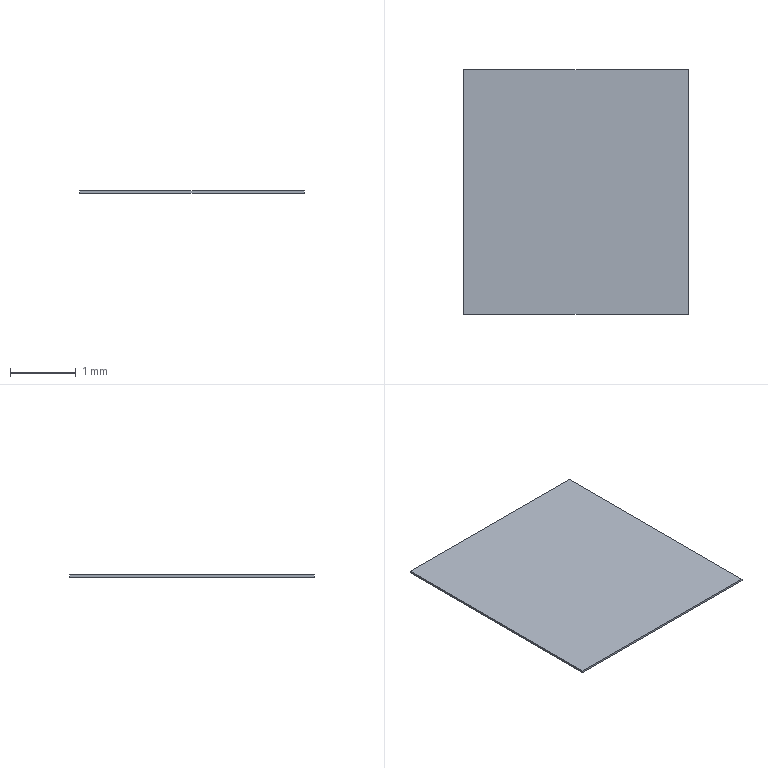Part | Creo | 1 solid | 6 faces | box 3.425 x 3.725 x 0.03048 mm | volume 0.389 mm3 | plane 6
STEP:
#1=CARTESIAN_POINT('',(0.,0.,0.));
#2=DIRECTION('',(0.,0.,1.));
#3=DIRECTION('',(1.,0.,0.));
#4=AXIS2_PLACEMENT_3D('',#1,#2,#3);
#5=CARTESIAN_POINT('',(-1.713,-1.863,0.));
#6=VERTEX_POINT('',#5);
#7=CARTESIAN_POINT('',(1.713,-1.863,0.));
#8=VERTEX_POINT('',#7);
#9=CARTESIAN_POINT('',(-1.713,-1.863,0.));
#10=DIRECTION('',(1.,0.,0.));
#11=VECTOR('',#10,3.425);
#12=LINE('',#9,#11);
#13=EDGE_CURVE('',#6,#8,#12,.T.);
#14=ORIENTED_EDGE('',*,*,#13,.T.);
#15=CARTESIAN_POINT('',(1.713,1.863,0.));
#16=VERTEX_POINT('',#15);
#17=CARTESIAN_POINT('',(1.713,-1.863,0.));
#18=DIRECTION('',(0.,1.,0.));
#19=VECTOR('',#18,3.725);
#20=LINE('',#17,#19);
#21=EDGE_CURVE('',#8,#16,#20,.T.);
#22=ORIENTED_EDGE('',*,*,#21,.T.);
#23=CARTESIAN_POINT('',(-1.713,1.863,0.));
#24=VERTEX_POINT('',#23);
#25=CARTESIAN_POINT('',(1.713,1.863,0.));
#26=DIRECTION('',(-1.,0.,0.));
#27=VECTOR('',#26,3.425);
#28=LINE('',#25,#27);
#29=EDGE_CURVE('',#16,#24,#28,.T.);
#30=ORIENTED_EDGE('',*,*,#29,.T.);
#31=CARTESIAN_POINT('',(-1.713,1.863,0.));
#32=DIRECTION('',(0.,-1.,0.));
#33=VECTOR('',#32,3.725);
#34=LINE('',#31,#33);
#35=EDGE_CURVE('',#24,#6,#34,.T.);
#36=ORIENTED_EDGE('',*,*,#35,.T.);
#37=EDGE_LOOP('',(#14,#22,#30,#36));
#38=FACE_OUTER_BOUND('',#37,.F.);
#39=CARTESIAN_POINT('',(0.,0.,0.));
#40=DIRECTION('',(0.,0.,1.));
#41=DIRECTION('',(1.,0.,0.));
#42=AXIS2_PLACEMENT_3D('',#39,#40,#41);
#43=PLANE('',#42);
#44=ADVANCED_FACE('',(#38),#43,.F.);
#45=ORIENTED_EDGE('',*,*,#13,.F.);
#46=CARTESIAN_POINT('',(-1.713,-1.863,0.03048));
#47=VERTEX_POINT('',#46);
#48=CARTESIAN_POINT('',(-1.713,-1.863,0.));
#49=DIRECTION('',(0.,0.,1.));
#50=VECTOR('',#49,0.03048);
#51=LINE('',#48,#50);
#52=EDGE_CURVE('',#6,#47,#51,.T.);
#53=ORIENTED_EDGE('',*,*,#52,.T.);
#54=CARTESIAN_POINT('',(1.713,-1.863,0.03048));
#55=VERTEX_POINT('',#54);
#56=CARTESIAN_POINT('',(-1.713,-1.863,0.03048));
#57=DIRECTION('',(1.,0.,0.));
#58=VECTOR('',#57,3.425);
#59=LINE('',#56,#58);
#60=EDGE_CURVE('',#47,#55,#59,.T.);
#61=ORIENTED_EDGE('',*,*,#60,.T.);
#62=CARTESIAN_POINT('',(1.713,-1.863,0.));
#63=DIRECTION('',(0.,0.,1.));
#64=VECTOR('',#63,0.03048);
#65=LINE('',#62,#64);
#66=EDGE_CURVE('',#8,#55,#65,.T.);
#67=ORIENTED_EDGE('',*,*,#66,.F.);
#68=EDGE_LOOP('',(#45,#53,#61,#67));
#69=FACE_OUTER_BOUND('',#68,.F.);
#70=CARTESIAN_POINT('',(-1.713,-1.863,0.));
#71=DIRECTION('',(0.,-1.,0.));
#72=DIRECTION('',(1.,0.,0.));
#73=AXIS2_PLACEMENT_3D('',#70,#71,#72);
#74=PLANE('',#73);
#75=ADVANCED_FACE('',(#69),#74,.T.);
#76=ORIENTED_EDGE('',*,*,#35,.F.);
#77=CARTESIAN_POINT('',(-1.713,1.863,0.03048));
#78=VERTEX_POINT('',#77);
#79=CARTESIAN_POINT('',(-1.713,1.863,0.));
#80=DIRECTION('',(0.,0.,1.));
#81=VECTOR('',#80,0.03048);
#82=LINE('',#79,#81);
#83=EDGE_CURVE('',#24,#78,#82,.T.);
#84=ORIENTED_EDGE('',*,*,#83,.T.);
#85=CARTESIAN_POINT('',(-1.713,1.863,0.03048));
#86=DIRECTION('',(0.,-1.,0.));
#87=VECTOR('',#86,3.725);
#88=LINE('',#85,#87);
#89=EDGE_CURVE('',#78,#47,#88,.T.);
#90=ORIENTED_EDGE('',*,*,#89,.T.);
#91=ORIENTED_EDGE('',*,*,#52,.F.);
#92=EDGE_LOOP('',(#76,#84,#90,#91));
#93=FACE_OUTER_BOUND('',#92,.F.);
#94=CARTESIAN_POINT('',(-1.713,1.863,0.));
#95=DIRECTION('',(-1.,0.,0.));
#96=DIRECTION('',(0.,-1.,0.));
#97=AXIS2_PLACEMENT_3D('',#94,#95,#96);
#98=PLANE('',#97);
#99=ADVANCED_FACE('',(#93),#98,.T.);
#100=ORIENTED_EDGE('',*,*,#29,.F.);
#101=CARTESIAN_POINT('',(1.713,1.863,0.03048));
#102=VERTEX_POINT('',#101);
#103=CARTESIAN_POINT('',(1.713,1.863,0.));
#104=DIRECTION('',(0.,0.,1.));
#105=VECTOR('',#104,0.03048);
#106=LINE('',#103,#105);
#107=EDGE_CURVE('',#16,#102,#106,.T.);
#108=ORIENTED_EDGE('',*,*,#107,.T.);
#109=CARTESIAN_POINT('',(1.713,1.863,0.03048));
#110=DIRECTION('',(-1.,0.,0.));
#111=VECTOR('',#110,3.425);
#112=LINE('',#109,#111);
#113=EDGE_CURVE('',#102,#78,#112,.T.);
#114=ORIENTED_EDGE('',*,*,#113,.T.);
#115=ORIENTED_EDGE('',*,*,#83,.F.);
#116=EDGE_LOOP('',(#100,#108,#114,#115));
#117=FACE_OUTER_BOUND('',#116,.F.);
#118=CARTESIAN_POINT('',(1.713,1.863,0.));
#119=DIRECTION('',(0.,1.,0.));
#120=DIRECTION('',(-1.,0.,0.));
#121=AXIS2_PLACEMENT_3D('',#118,#119,#120);
#122=PLANE('',#121);
#123=ADVANCED_FACE('',(#117),#122,.T.);
#124=ORIENTED_EDGE('',*,*,#21,.F.);
#125=ORIENTED_EDGE('',*,*,#66,.T.);
#126=CARTESIAN_POINT('',(1.713,-1.863,0.03048));
#127=DIRECTION('',(0.,1.,0.));
#128=VECTOR('',#127,3.725);
#129=LINE('',#126,#128);
#130=EDGE_CURVE('',#55,#102,#129,.T.);
#131=ORIENTED_EDGE('',*,*,#130,.T.);
#132=ORIENTED_EDGE('',*,*,#107,.F.);
#133=EDGE_LOOP('',(#124,#125,#131,#132));
#134=FACE_OUTER_BOUND('',#133,.F.);
#135=CARTESIAN_POINT('',(1.713,-1.863,0.));
#136=DIRECTION('',(1.,0.,0.));
#137=DIRECTION('',(0.,1.,0.));
#138=AXIS2_PLACEMENT_3D('',#135,#136,#137);
#139=PLANE('',#138);
#140=ADVANCED_FACE('',(#134),#139,.T.);
#141=ORIENTED_EDGE('',*,*,#60,.F.);
#142=ORIENTED_EDGE('',*,*,#89,.F.);
#143=ORIENTED_EDGE('',*,*,#113,.F.);
#144=ORIENTED_EDGE('',*,*,#130,.F.);
#145=EDGE_LOOP('',(#141,#142,#143,#144));
#146=FACE_OUTER_BOUND('',#145,.F.);
#147=CARTESIAN_POINT('',(0.,0.,0.03048));
#148=DIRECTION('',(0.,0.,1.));
#149=DIRECTION('',(1.,0.,0.));
#150=AXIS2_PLACEMENT_3D('',#147,#148,#149);
#151=PLANE('',#150);
#152=ADVANCED_FACE('',(#146),#151,.T.);
#153=CLOSED_SHELL('',(#44,#75,#99,#123,#140,#152));
#154=MANIFOLD_SOLID_BREP('',#153);
#155=(LENGTH_UNIT()NAMED_UNIT(*)SI_UNIT(.MILLI.,.METRE.));
#156=UNCERTAINTY_MEASURE_WITH_UNIT(LENGTH_MEASURE(0.0005061),#155,'','');
#157=(NAMED_UNIT(*)PLANE_ANGLE_UNIT()SI_UNIT($,.RADIAN.));
#158=PLANE_ANGLE_MEASURE_WITH_UNIT(PLANE_ANGLE_MEASURE(0.01745),#157);
#159=(CONVERSION_BASED_UNIT('DEGREE',#158)NAMED_UNIT(*)PLANE_ANGLE_UNIT());
#160=(NAMED_UNIT(*)SI_UNIT($,.STERADIAN.)SOLID_ANGLE_UNIT());
#161=(GEOMETRIC_REPRESENTATION_CONTEXT(3)GLOBAL_UNCERTAINTY_ASSIGNED_CONTEXT((#156))GLOBAL_UNIT_ASSIGNED_CONTEXT((#155,#159,#160))REPRESENTATION_CONTEXT('',''));
#162=ADVANCED_BREP_SHAPE_REPRESENTATION('',(#4,#154),#161);